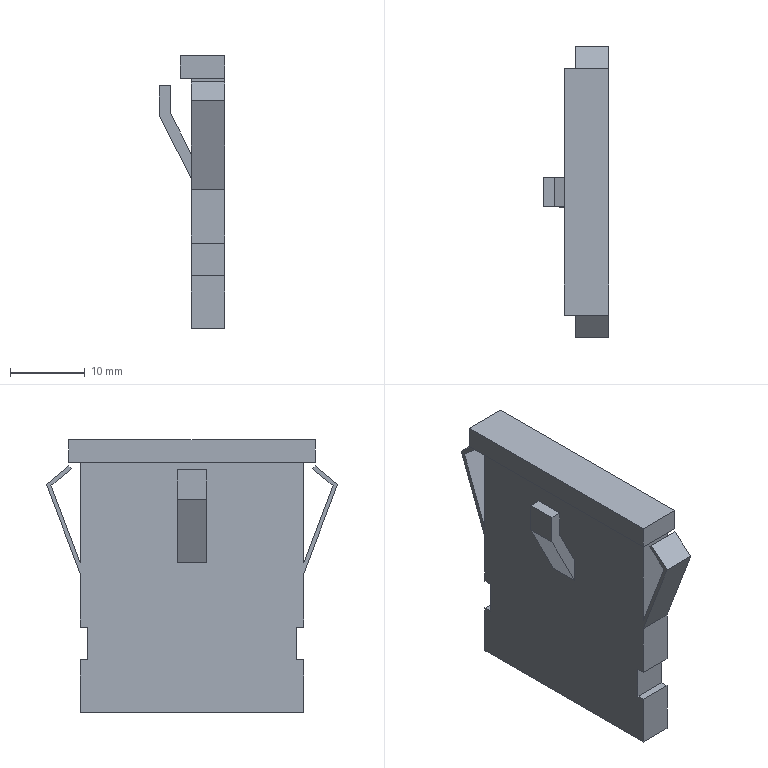Part | STEP file | A7P_M_LEFT | 1 solid | 37 faces | box 8.8 x 39 x 36.5 mm | volume 5217 mm3 | plane 37
STEP:
#1=CARTESIAN_POINT('',(0.,-15.,-26.5));
#2=VERTEX_POINT('',#1);
#3=CARTESIAN_POINT('',(-4.5,-15.,-26.5));
#4=VERTEX_POINT('',#3);
#5=CARTESIAN_POINT('',(0.,-15.,-26.5));
#6=DIRECTION('',(-1.,0.,0.));
#7=VECTOR('',#6,1000.);
#8=LINE('',#5,#7);
#9=EDGE_CURVE('',#2,#4,#8,.T.);
#10=ORIENTED_EDGE('',*,*,#9,.T.);
#11=CARTESIAN_POINT('',(-4.5,-15.,-33.5));
#12=VERTEX_POINT('',#11);
#13=CARTESIAN_POINT('',(-4.5,-15.,0.));
#14=DIRECTION('',(0.,0.,-1.));
#15=VECTOR('',#14,1000.);
#16=LINE('',#13,#15);
#17=EDGE_CURVE('',#4,#12,#16,.T.);
#18=ORIENTED_EDGE('',*,*,#17,.T.);
#19=CARTESIAN_POINT('',(0.,-15.,-33.5));
#20=VERTEX_POINT('',#19);
#21=CARTESIAN_POINT('',(-4.5,-15.,-33.5));
#22=DIRECTION('',(1.,0.,0.));
#23=VECTOR('',#22,1000.);
#24=LINE('',#21,#23);
#25=EDGE_CURVE('',#12,#20,#24,.T.);
#26=ORIENTED_EDGE('',*,*,#25,.T.);
#27=CARTESIAN_POINT('',(0.,-15.,0.));
#28=DIRECTION('',(0.,0.,-1.));
#29=VECTOR('',#28,1000.);
#30=LINE('',#27,#29);
#31=EDGE_CURVE('',#2,#20,#30,.T.);
#32=ORIENTED_EDGE('',*,*,#31,.F.);
#33=EDGE_LOOP('',(#10,#18,#26,#32));
#34=FACE_OUTER_BOUND('',#33,.T.);
#35=CARTESIAN_POINT('',(-4.5,-15.,0.));
#36=DIRECTION('',(0.,-1.,0.));
#37=DIRECTION('',(0.,0.,-1.));
#38=AXIS2_PLACEMENT_3D('',#35,#36,#37);
#39=PLANE('',#38);
#40=ADVANCED_FACE('',(#34),#39,.T.);
#41=CARTESIAN_POINT('',(0.,15.,-26.5));
#42=VERTEX_POINT('',#41);
#43=CARTESIAN_POINT('',(-4.5,15.,-26.5));
#44=VERTEX_POINT('',#43);
#45=CARTESIAN_POINT('',(0.,15.,-26.5));
#46=DIRECTION('',(-1.,0.,0.));
#47=VECTOR('',#46,1000.);
#48=LINE('',#45,#47);
#49=EDGE_CURVE('',#42,#44,#48,.T.);
#50=ORIENTED_EDGE('',*,*,#49,.F.);
#51=CARTESIAN_POINT('',(0.,15.,-33.5));
#52=VERTEX_POINT('',#51);
#53=CARTESIAN_POINT('',(0.,15.,0.));
#54=DIRECTION('',(0.,0.,1.));
#55=VECTOR('',#54,1000.);
#56=LINE('',#53,#55);
#57=EDGE_CURVE('',#52,#42,#56,.T.);
#58=ORIENTED_EDGE('',*,*,#57,.F.);
#59=CARTESIAN_POINT('',(-4.5,15.,-33.5));
#60=VERTEX_POINT('',#59);
#61=CARTESIAN_POINT('',(-4.5,15.,-33.5));
#62=DIRECTION('',(1.,0.,0.));
#63=VECTOR('',#62,1000.);
#64=LINE('',#61,#63);
#65=EDGE_CURVE('',#60,#52,#64,.T.);
#66=ORIENTED_EDGE('',*,*,#65,.F.);
#67=CARTESIAN_POINT('',(-4.5,15.,0.));
#68=DIRECTION('',(0.,0.,1.));
#69=VECTOR('',#68,1000.);
#70=LINE('',#67,#69);
#71=EDGE_CURVE('',#60,#44,#70,.T.);
#72=ORIENTED_EDGE('',*,*,#71,.T.);
#73=EDGE_LOOP('',(#50,#58,#66,#72));
#74=FACE_OUTER_BOUND('',#73,.T.);
#75=CARTESIAN_POINT('',(-4.5,15.,0.));
#76=DIRECTION('',(0.,1.,0.));
#77=DIRECTION('',(0.,0.,1.));
#78=AXIS2_PLACEMENT_3D('',#75,#76,#77);
#79=PLANE('',#78);
#80=ADVANCED_FACE('',(#74),#79,.T.);
#81=CARTESIAN_POINT('',(0.,-15.,-22.1));
#82=VERTEX_POINT('',#81);
#83=CARTESIAN_POINT('',(-4.5,-15.,-22.1));
#84=VERTEX_POINT('',#83);
#85=CARTESIAN_POINT('',(0.,-15.,-22.1));
#86=DIRECTION('',(-1.,0.,0.));
#87=VECTOR('',#86,1000.);
#88=LINE('',#85,#87);
#89=EDGE_CURVE('',#82,#84,#88,.T.);
#90=ORIENTED_EDGE('',*,*,#89,.F.);
#91=CARTESIAN_POINT('',(0.,-15.,-14.9));
#92=VERTEX_POINT('',#91);
#93=CARTESIAN_POINT('',(0.,-15.,0.));
#94=DIRECTION('',(0.,0.,-1.));
#95=VECTOR('',#94,1000.);
#96=LINE('',#93,#95);
#97=EDGE_CURVE('',#92,#82,#96,.T.);
#98=ORIENTED_EDGE('',*,*,#97,.F.);
#99=CARTESIAN_POINT('',(-4.5,-15.,-14.9));
#100=VERTEX_POINT('',#99);
#101=CARTESIAN_POINT('',(0.,-15.,-14.9));
#102=DIRECTION('',(-1.,0.,0.));
#103=VECTOR('',#102,1000.);
#104=LINE('',#101,#103);
#105=EDGE_CURVE('',#92,#100,#104,.T.);
#106=ORIENTED_EDGE('',*,*,#105,.T.);
#107=CARTESIAN_POINT('',(-4.5,-15.,0.));
#108=DIRECTION('',(0.,0.,-1.));
#109=VECTOR('',#108,1000.);
#110=LINE('',#107,#109);
#111=EDGE_CURVE('',#100,#84,#110,.T.);
#112=ORIENTED_EDGE('',*,*,#111,.T.);
#113=EDGE_LOOP('',(#90,#98,#106,#112));
#114=FACE_OUTER_BOUND('',#113,.T.);
#115=CARTESIAN_POINT('',(-4.5,-15.,0.));
#116=DIRECTION('',(0.,-1.,0.));
#117=DIRECTION('',(0.,0.,-1.));
#118=AXIS2_PLACEMENT_3D('',#115,#116,#117);
#119=PLANE('',#118);
#120=ADVANCED_FACE('',(#114),#119,.T.);
#121=CARTESIAN_POINT('',(0.,15.,-22.1));
#122=VERTEX_POINT('',#121);
#123=CARTESIAN_POINT('',(-4.5,15.,-22.1));
#124=VERTEX_POINT('',#123);
#125=CARTESIAN_POINT('',(0.,15.,-22.1));
#126=DIRECTION('',(-1.,0.,0.));
#127=VECTOR('',#126,1000.);
#128=LINE('',#125,#127);
#129=EDGE_CURVE('',#122,#124,#128,.T.);
#130=ORIENTED_EDGE('',*,*,#129,.T.);
#131=CARTESIAN_POINT('',(-4.5,15.,-14.9));
#132=VERTEX_POINT('',#131);
#133=CARTESIAN_POINT('',(-4.5,15.,0.));
#134=DIRECTION('',(0.,0.,1.));
#135=VECTOR('',#134,1000.);
#136=LINE('',#133,#135);
#137=EDGE_CURVE('',#124,#132,#136,.T.);
#138=ORIENTED_EDGE('',*,*,#137,.T.);
#139=CARTESIAN_POINT('',(0.,15.,-14.9));
#140=VERTEX_POINT('',#139);
#141=CARTESIAN_POINT('',(0.,15.,-14.9));
#142=DIRECTION('',(-1.,0.,0.));
#143=VECTOR('',#142,1000.);
#144=LINE('',#141,#143);
#145=EDGE_CURVE('',#140,#132,#144,.T.);
#146=ORIENTED_EDGE('',*,*,#145,.F.);
#147=CARTESIAN_POINT('',(0.,15.,0.));
#148=DIRECTION('',(0.,0.,1.));
#149=VECTOR('',#148,1000.);
#150=LINE('',#147,#149);
#151=EDGE_CURVE('',#122,#140,#150,.T.);
#152=ORIENTED_EDGE('',*,*,#151,.F.);
#153=EDGE_LOOP('',(#130,#138,#146,#152));
#154=FACE_OUTER_BOUND('',#153,.T.);
#155=CARTESIAN_POINT('',(-4.5,15.,0.));
#156=DIRECTION('',(0.,1.,0.));
#157=DIRECTION('',(0.,0.,1.));
#158=AXIS2_PLACEMENT_3D('',#155,#156,#157);
#159=PLANE('',#158);
#160=ADVANCED_FACE('',(#154),#159,.T.);
#161=CARTESIAN_POINT('',(0.,15.,-13.486));
#162=VERTEX_POINT('',#161);
#163=CARTESIAN_POINT('',(-4.5,15.,-13.486));
#164=VERTEX_POINT('',#163);
#165=CARTESIAN_POINT('',(0.,15.,-13.486));
#166=DIRECTION('',(-1.,0.,0.));
#167=VECTOR('',#166,1000.);
#168=LINE('',#165,#167);
#169=EDGE_CURVE('',#162,#164,#168,.T.);
#170=ORIENTED_EDGE('',*,*,#169,.T.);
#171=CARTESIAN_POINT('',(-4.5,15.,0.));
#172=VERTEX_POINT('',#171);
#173=CARTESIAN_POINT('',(-4.5,15.,0.));
#174=DIRECTION('',(0.,0.,1.));
#175=VECTOR('',#174,1000.);
#176=LINE('',#173,#175);
#177=EDGE_CURVE('',#164,#172,#176,.T.);
#178=ORIENTED_EDGE('',*,*,#177,.T.);
#179=CARTESIAN_POINT('',(0.,15.,0.));
#180=VERTEX_POINT('',#179);
#181=CARTESIAN_POINT('',(-4.5,15.,0.));
#182=DIRECTION('',(1.,0.,0.));
#183=VECTOR('',#182,1000.);
#184=LINE('',#181,#183);
#185=EDGE_CURVE('',#172,#180,#184,.T.);
#186=ORIENTED_EDGE('',*,*,#185,.T.);
#187=CARTESIAN_POINT('',(0.,15.,0.));
#188=DIRECTION('',(0.,0.,1.));
#189=VECTOR('',#188,1000.);
#190=LINE('',#187,#189);
#191=EDGE_CURVE('',#162,#180,#190,.T.);
#192=ORIENTED_EDGE('',*,*,#191,.F.);
#193=EDGE_LOOP('',(#170,#178,#186,#192));
#194=FACE_OUTER_BOUND('',#193,.T.);
#195=CARTESIAN_POINT('',(-4.5,15.,0.));
#196=DIRECTION('',(0.,1.,0.));
#197=DIRECTION('',(0.,0.,1.));
#198=AXIS2_PLACEMENT_3D('',#195,#196,#197);
#199=PLANE('',#198);
#200=ADVANCED_FACE('',(#194),#199,.T.);
#201=CARTESIAN_POINT('',(0.,15.,-33.5));
#202=DIRECTION('',(0.,1.,0.));
#203=VECTOR('',#202,1000.);
#204=LINE('',#201,#203);
#205=EDGE_CURVE('',#20,#52,#204,.T.);
#206=ORIENTED_EDGE('',*,*,#205,.F.);
#207=ORIENTED_EDGE('',*,*,#25,.F.);
#208=CARTESIAN_POINT('',(-4.5,15.,-33.5));
#209=DIRECTION('',(0.,1.,0.));
#210=VECTOR('',#209,1000.);
#211=LINE('',#208,#210);
#212=EDGE_CURVE('',#12,#60,#211,.T.);
#213=ORIENTED_EDGE('',*,*,#212,.T.);
#214=ORIENTED_EDGE('',*,*,#65,.T.);
#215=EDGE_LOOP('',(#206,#207,#213,#214));
#216=FACE_OUTER_BOUND('',#215,.T.);
#217=CARTESIAN_POINT('',(-4.5,15.,-33.5));
#218=DIRECTION('',(0.,0.,-1.));
#219=DIRECTION('',(-1.,0.,0.));
#220=AXIS2_PLACEMENT_3D('',#217,#218,#219);
#221=PLANE('',#220);
#222=ADVANCED_FACE('',(#216),#221,.T.);
#223=CARTESIAN_POINT('',(0.,-15.,-13.486));
#224=VERTEX_POINT('',#223);
#225=CARTESIAN_POINT('',(-4.5,-15.,-13.486));
#226=VERTEX_POINT('',#225);
#227=CARTESIAN_POINT('',(0.,-15.,-13.486));
#228=DIRECTION('',(-1.,0.,0.));
#229=VECTOR('',#228,1000.);
#230=LINE('',#227,#229);
#231=EDGE_CURVE('',#224,#226,#230,.T.);
#232=ORIENTED_EDGE('',*,*,#231,.F.);
#233=CARTESIAN_POINT('',(0.,-15.,0.));
#234=VERTEX_POINT('',#233);
#235=CARTESIAN_POINT('',(0.,-15.,0.));
#236=DIRECTION('',(0.,0.,-1.));
#237=VECTOR('',#236,1000.);
#238=LINE('',#235,#237);
#239=EDGE_CURVE('',#234,#224,#238,.T.);
#240=ORIENTED_EDGE('',*,*,#239,.F.);
#241=CARTESIAN_POINT('',(-4.5,-15.,0.));
#242=VERTEX_POINT('',#241);
#243=CARTESIAN_POINT('',(-4.5,-15.,0.));
#244=DIRECTION('',(1.,0.,0.));
#245=VECTOR('',#244,1000.);
#246=LINE('',#243,#245);
#247=EDGE_CURVE('',#242,#234,#246,.T.);
#248=ORIENTED_EDGE('',*,*,#247,.F.);
#249=CARTESIAN_POINT('',(-4.5,-15.,0.));
#250=DIRECTION('',(0.,0.,-1.));
#251=VECTOR('',#250,1000.);
#252=LINE('',#249,#251);
#253=EDGE_CURVE('',#242,#226,#252,.T.);
#254=ORIENTED_EDGE('',*,*,#253,.T.);
#255=EDGE_LOOP('',(#232,#240,#248,#254));
#256=FACE_OUTER_BOUND('',#255,.T.);
#257=CARTESIAN_POINT('',(-4.5,-15.,0.));
#258=DIRECTION('',(0.,-1.,0.));
#259=DIRECTION('',(0.,0.,-1.));
#260=AXIS2_PLACEMENT_3D('',#257,#258,#259);
#261=PLANE('',#260);
#262=ADVANCED_FACE('',(#256),#261,.T.);
#263=CARTESIAN_POINT('',(0.,-16.5,0.));
#264=VERTEX_POINT('',#263);
#265=CARTESIAN_POINT('',(0.,-16.5,0.));
#266=DIRECTION('',(0.,1.,0.));
#267=VECTOR('',#266,1000.);
#268=LINE('',#265,#267);
#269=EDGE_CURVE('',#264,#234,#268,.T.);
#270=ORIENTED_EDGE('',*,*,#269,.F.);
#271=CARTESIAN_POINT('',(-6.,-16.5,0.));
#272=VERTEX_POINT('',#271);
#273=CARTESIAN_POINT('',(-4.5,-16.5,0.));
#274=DIRECTION('',(1.,0.,0.));
#275=VECTOR('',#274,1000.);
#276=LINE('',#273,#275);
#277=EDGE_CURVE('',#272,#264,#276,.T.);
#278=ORIENTED_EDGE('',*,*,#277,.F.);
#279=CARTESIAN_POINT('',(-6.,16.5,0.));
#280=VERTEX_POINT('',#279);
#281=CARTESIAN_POINT('',(-6.,16.5,0.));
#282=DIRECTION('',(0.,-1.,0.));
#283=VECTOR('',#282,1000.);
#284=LINE('',#281,#283);
#285=EDGE_CURVE('',#280,#272,#284,.T.);
#286=ORIENTED_EDGE('',*,*,#285,.F.);
#287=CARTESIAN_POINT('',(0.,16.5,0.));
#288=VERTEX_POINT('',#287);
#289=CARTESIAN_POINT('',(-4.5,16.5,0.));
#290=DIRECTION('',(1.,0.,0.));
#291=VECTOR('',#290,1000.);
#292=LINE('',#289,#291);
#293=EDGE_CURVE('',#280,#288,#292,.T.);
#294=ORIENTED_EDGE('',*,*,#293,.T.);
#295=CARTESIAN_POINT('',(0.,15.,0.));
#296=DIRECTION('',(0.,1.,0.));
#297=VECTOR('',#296,1000.);
#298=LINE('',#295,#297);
#299=EDGE_CURVE('',#180,#288,#298,.T.);
#300=ORIENTED_EDGE('',*,*,#299,.F.);
#301=ORIENTED_EDGE('',*,*,#185,.F.);
#302=CARTESIAN_POINT('',(-4.5,16.5,0.));
#303=DIRECTION('',(0.,1.,0.));
#304=VECTOR('',#303,1000.);
#305=LINE('',#302,#304);
#306=EDGE_CURVE('',#242,#172,#305,.T.);
#307=ORIENTED_EDGE('',*,*,#306,.F.);
#308=ORIENTED_EDGE('',*,*,#247,.T.);
#309=EDGE_LOOP('',(#270,#278,#286,#294,#300,#301,#307,#308));
#310=FACE_OUTER_BOUND('',#309,.T.);
#311=CARTESIAN_POINT('',(-4.5,-16.5,0.));
#312=DIRECTION('',(0.,0.,-1.));
#313=DIRECTION('',(-1.,0.,0.));
#314=AXIS2_PLACEMENT_3D('',#311,#312,#313);
#315=PLANE('',#314);
#316=ADVANCED_FACE('',(#310),#315,.T.);
#317=CARTESIAN_POINT('',(0.,-16.5,3.));
#318=VERTEX_POINT('',#317);
#319=CARTESIAN_POINT('',(0.,-16.5,3.));
#320=DIRECTION('',(0.,0.,-1.));
#321=VECTOR('',#320,1000.);
#322=LINE('',#319,#321);
#323=EDGE_CURVE('',#318,#264,#322,.T.);
#324=ORIENTED_EDGE('',*,*,#323,.F.);
#325=CARTESIAN_POINT('',(-6.,-16.5,3.));
#326=VERTEX_POINT('',#325);
#327=CARTESIAN_POINT('',(-4.5,-16.5,3.));
#328=DIRECTION('',(1.,0.,0.));
#329=VECTOR('',#328,1000.);
#330=LINE('',#327,#329);
#331=EDGE_CURVE('',#326,#318,#330,.T.);
#332=ORIENTED_EDGE('',*,*,#331,.F.);
#333=CARTESIAN_POINT('',(-6.,-16.5,-33.541));
#334=DIRECTION('',(0.,0.,1.));
#335=VECTOR('',#334,1000.);
#336=LINE('',#333,#335);
#337=EDGE_CURVE('',#272,#326,#336,.T.);
#338=ORIENTED_EDGE('',*,*,#337,.F.);
#339=ORIENTED_EDGE('',*,*,#277,.T.);
#340=EDGE_LOOP('',(#324,#332,#338,#339));
#341=FACE_OUTER_BOUND('',#340,.T.);
#342=CARTESIAN_POINT('',(-4.5,-16.5,3.));
#343=DIRECTION('',(0.,-1.,0.));
#344=DIRECTION('',(0.,0.,-1.));
#345=AXIS2_PLACEMENT_3D('',#342,#343,#344);
#346=PLANE('',#345);
#347=ADVANCED_FACE('',(#341),#346,.T.);
#348=CARTESIAN_POINT('',(0.,16.5,3.));
#349=VERTEX_POINT('',#348);
#350=CARTESIAN_POINT('',(0.,16.5,3.));
#351=DIRECTION('',(0.,-1.,0.));
#352=VECTOR('',#351,1000.);
#353=LINE('',#350,#352);
#354=EDGE_CURVE('',#349,#318,#353,.T.);
#355=ORIENTED_EDGE('',*,*,#354,.F.);
#356=CARTESIAN_POINT('',(-6.,16.5,3.));
#357=VERTEX_POINT('',#356);
#358=CARTESIAN_POINT('',(-4.5,16.5,3.));
#359=DIRECTION('',(1.,0.,0.));
#360=VECTOR('',#359,1000.);
#361=LINE('',#358,#360);
#362=EDGE_CURVE('',#357,#349,#361,.T.);
#363=ORIENTED_EDGE('',*,*,#362,.F.);
#364=CARTESIAN_POINT('',(-6.,16.5,3.));
#365=DIRECTION('',(0.,-1.,0.));
#366=VECTOR('',#365,1000.);
#367=LINE('',#364,#366);
#368=EDGE_CURVE('',#357,#326,#367,.T.);
#369=ORIENTED_EDGE('',*,*,#368,.T.);
#370=ORIENTED_EDGE('',*,*,#331,.T.);
#371=EDGE_LOOP('',(#355,#363,#369,#370));
#372=FACE_OUTER_BOUND('',#371,.T.);
#373=CARTESIAN_POINT('',(-4.5,16.5,3.));
#374=DIRECTION('',(0.,0.,1.));
#375=DIRECTION('',(1.,0.,0.));
#376=AXIS2_PLACEMENT_3D('',#373,#374,#375);
#377=PLANE('',#376);
#378=ADVANCED_FACE('',(#372),#377,.T.);
#379=CARTESIAN_POINT('',(0.,16.5,0.));
#380=DIRECTION('',(0.,0.,1.));
#381=VECTOR('',#380,1000.);
#382=LINE('',#379,#381);
#383=EDGE_CURVE('',#288,#349,#382,.T.);
#384=ORIENTED_EDGE('',*,*,#383,.F.);
#385=ORIENTED_EDGE('',*,*,#293,.F.);
#386=CARTESIAN_POINT('',(-6.,16.5,-33.541));
#387=DIRECTION('',(0.,0.,1.));
#388=VECTOR('',#387,1000.);
#389=LINE('',#386,#388);
#390=EDGE_CURVE('',#280,#357,#389,.T.);
#391=ORIENTED_EDGE('',*,*,#390,.T.);
#392=ORIENTED_EDGE('',*,*,#362,.T.);
#393=EDGE_LOOP('',(#384,#385,#391,#392));
#394=FACE_OUTER_BOUND('',#393,.T.);
#395=CARTESIAN_POINT('',(-4.5,16.5,0.));
#396=DIRECTION('',(0.,1.,0.));
#397=DIRECTION('',(0.,0.,1.));
#398=AXIS2_PLACEMENT_3D('',#395,#396,#397);
#399=PLANE('',#398);
#400=ADVANCED_FACE('',(#394),#399,.T.);
#401=CARTESIAN_POINT('',(-4.5,2.,-13.5));
#402=VERTEX_POINT('',#401);
#403=CARTESIAN_POINT('',(-4.5,-2.,-13.5));
#404=VERTEX_POINT('',#403);
#405=CARTESIAN_POINT('',(-4.5,2.,-13.5));
#406=DIRECTION('',(0.,-1.,0.));
#407=VECTOR('',#406,1000.);
#408=LINE('',#405,#407);
#409=EDGE_CURVE('',#402,#404,#408,.T.);
#410=ORIENTED_EDGE('',*,*,#409,.F.);
#411=CARTESIAN_POINT('',(-4.5,2.,-10.177));
#412=VERTEX_POINT('',#411);
#413=CARTESIAN_POINT('',(-4.5,2.,-13.5));
#414=DIRECTION('',(0.,0.,-1.));
#415=VECTOR('',#414,1000.);
#416=LINE('',#413,#415);
#417=EDGE_CURVE('',#412,#402,#416,.T.);
#418=ORIENTED_EDGE('',*,*,#417,.F.);
#419=CARTESIAN_POINT('',(-4.5,-2.,-10.177));
#420=VERTEX_POINT('',#419);
#421=CARTESIAN_POINT('',(-4.5,2.,-10.177));
#422=DIRECTION('',(0.,-1.,0.));
#423=VECTOR('',#422,1000.);
#424=LINE('',#421,#423);
#425=EDGE_CURVE('',#412,#420,#424,.T.);
#426=ORIENTED_EDGE('',*,*,#425,.T.);
#427=CARTESIAN_POINT('',(-4.5,-2.,-13.5));
#428=DIRECTION('',(0.,0.,-1.));
#429=VECTOR('',#428,1000.);
#430=LINE('',#427,#429);
#431=EDGE_CURVE('',#420,#404,#430,.T.);
#432=ORIENTED_EDGE('',*,*,#431,.T.);
#433=EDGE_LOOP('',(#410,#418,#426,#432));
#434=FACE_BOUND('',#433,.T.);
#435=ORIENTED_EDGE('',*,*,#17,.F.);
#436=CARTESIAN_POINT('',(-4.5,-14.,-26.5));
#437=VERTEX_POINT('',#436);
#438=CARTESIAN_POINT('',(-4.5,-15.,-26.5));
#439=DIRECTION('',(0.,-1.,0.));
#440=VECTOR('',#439,1000.);
#441=LINE('',#438,#440);
#442=EDGE_CURVE('',#437,#4,#441,.T.);
#443=ORIENTED_EDGE('',*,*,#442,.F.);
#444=CARTESIAN_POINT('',(-4.5,-14.,-22.1));
#445=VERTEX_POINT('',#444);
#446=CARTESIAN_POINT('',(-4.5,-14.,-26.5));
#447=DIRECTION('',(0.,0.,-1.));
#448=VECTOR('',#447,1000.);
#449=LINE('',#446,#448);
#450=EDGE_CURVE('',#445,#437,#449,.T.);
#451=ORIENTED_EDGE('',*,*,#450,.F.);
#452=CARTESIAN_POINT('',(-4.5,-15.,-22.1));
#453=DIRECTION('',(0.,1.,0.));
#454=VECTOR('',#453,1000.);
#455=LINE('',#452,#454);
#456=EDGE_CURVE('',#84,#445,#455,.T.);
#457=ORIENTED_EDGE('',*,*,#456,.F.);
#458=ORIENTED_EDGE('',*,*,#111,.F.);
#459=CARTESIAN_POINT('',(-4.5,-19.5,-3.));
#460=VERTEX_POINT('',#459);
#461=CARTESIAN_POINT('',(-4.5,-15.,-14.9));
#462=DIRECTION('',(0.,-0.3537,0.9354));
#463=VECTOR('',#462,1000.);
#464=LINE('',#461,#463);
#465=EDGE_CURVE('',#100,#460,#464,.T.);
#466=ORIENTED_EDGE('',*,*,#465,.T.);
#467=CARTESIAN_POINT('',(-4.5,-16.5,-0.5));
#468=VERTEX_POINT('',#467);
#469=CARTESIAN_POINT('',(-4.5,-19.5,-3.));
#470=DIRECTION('',(0.,0.7682,0.6402));
#471=VECTOR('',#470,1000.);
#472=LINE('',#469,#471);
#473=EDGE_CURVE('',#460,#468,#472,.T.);
#474=ORIENTED_EDGE('',*,*,#473,.T.);
#475=CARTESIAN_POINT('',(-4.5,-16.18,-0.8841));
#476=VERTEX_POINT('',#475);
#477=CARTESIAN_POINT('',(-4.5,-16.5,-0.5));
#478=DIRECTION('',(0.,0.6402,-0.7682));
#479=VECTOR('',#478,1000.);
#480=LINE('',#477,#479);
#481=EDGE_CURVE('',#468,#476,#480,.T.);
#482=ORIENTED_EDGE('',*,*,#481,.T.);
#483=CARTESIAN_POINT('',(-4.5,-18.906,-3.156));
#484=VERTEX_POINT('',#483);
#485=CARTESIAN_POINT('',(-4.5,-18.906,-3.156));
#486=DIRECTION('',(0.,-0.7682,-0.6402));
#487=VECTOR('',#486,1000.);
#488=LINE('',#485,#487);
#489=EDGE_CURVE('',#476,#484,#488,.T.);
#490=ORIENTED_EDGE('',*,*,#489,.T.);
#491=CARTESIAN_POINT('',(-4.5,-15.,-13.486));
#492=DIRECTION('',(0.,0.3537,-0.9354));
#493=VECTOR('',#492,1000.);
#494=LINE('',#491,#493);
#495=EDGE_CURVE('',#484,#226,#494,.T.);
#496=ORIENTED_EDGE('',*,*,#495,.T.);
#497=ORIENTED_EDGE('',*,*,#253,.F.);
#498=ORIENTED_EDGE('',*,*,#306,.T.);
#499=ORIENTED_EDGE('',*,*,#177,.F.);
#500=CARTESIAN_POINT('',(-4.5,18.906,-3.156));
#501=VERTEX_POINT('',#500);
#502=CARTESIAN_POINT('',(-4.5,15.,-13.486));
#503=DIRECTION('',(0.,0.3537,0.9354));
#504=VECTOR('',#503,1000.);
#505=LINE('',#502,#504);
#506=EDGE_CURVE('',#164,#501,#505,.T.);
#507=ORIENTED_EDGE('',*,*,#506,.T.);
#508=CARTESIAN_POINT('',(-4.5,16.18,-0.8841));
#509=VERTEX_POINT('',#508);
#510=CARTESIAN_POINT('',(-4.5,18.906,-3.156));
#511=DIRECTION('',(0.,-0.7682,0.6402));
#512=VECTOR('',#511,1000.);
#513=LINE('',#510,#512);
#514=EDGE_CURVE('',#501,#509,#513,.T.);
#515=ORIENTED_EDGE('',*,*,#514,.T.);
#516=CARTESIAN_POINT('',(-4.5,16.5,-0.5));
#517=VERTEX_POINT('',#516);
#518=CARTESIAN_POINT('',(-4.5,16.5,-0.5));
#519=DIRECTION('',(0.,0.6402,0.7682));
#520=VECTOR('',#519,1000.);
#521=LINE('',#518,#520);
#522=EDGE_CURVE('',#509,#517,#521,.T.);
#523=ORIENTED_EDGE('',*,*,#522,.T.);
#524=CARTESIAN_POINT('',(-4.5,19.5,-3.));
#525=VERTEX_POINT('',#524);
#526=CARTESIAN_POINT('',(-4.5,19.5,-3.));
#527=DIRECTION('',(0.,0.7682,-0.6402));
#528=VECTOR('',#527,1000.);
#529=LINE('',#526,#528);
#530=EDGE_CURVE('',#517,#525,#529,.T.);
#531=ORIENTED_EDGE('',*,*,#530,.T.);
#532=CARTESIAN_POINT('',(-4.5,15.,-14.9));
#533=DIRECTION('',(0.,-0.3537,-0.9354));
#534=VECTOR('',#533,1000.);
#535=LINE('',#532,#534);
#536=EDGE_CURVE('',#525,#132,#535,.T.);
#537=ORIENTED_EDGE('',*,*,#536,.T.);
#538=ORIENTED_EDGE('',*,*,#137,.F.);
#539=CARTESIAN_POINT('',(-4.5,14.,-22.1));
#540=VERTEX_POINT('',#539);
#541=CARTESIAN_POINT('',(-4.5,15.,-22.1));
#542=DIRECTION('',(0.,1.,0.));
#543=VECTOR('',#542,1000.);
#544=LINE('',#541,#543);
#545=EDGE_CURVE('',#540,#124,#544,.T.);
#546=ORIENTED_EDGE('',*,*,#545,.F.);
#547=CARTESIAN_POINT('',(-4.5,14.,-26.5));
#548=VERTEX_POINT('',#547);
#549=CARTESIAN_POINT('',(-4.5,14.,-26.5));
#550=DIRECTION('',(0.,0.,1.));
#551=VECTOR('',#550,1000.);
#552=LINE('',#549,#551);
#553=EDGE_CURVE('',#548,#540,#552,.T.);
#554=ORIENTED_EDGE('',*,*,#553,.F.);
#555=CARTESIAN_POINT('',(-4.5,15.,-26.5));
#556=DIRECTION('',(0.,-1.,0.));
#557=VECTOR('',#556,1000.);
#558=LINE('',#555,#557);
#559=EDGE_CURVE('',#44,#548,#558,.T.);
#560=ORIENTED_EDGE('',*,*,#559,.F.);
#561=ORIENTED_EDGE('',*,*,#71,.F.);
#562=ORIENTED_EDGE('',*,*,#212,.F.);
#563=EDGE_LOOP('',(#435,#443,#451,#457,#458,#466,#474,#482,#490,#496,#497,#498,#499,#507,#515,#523,#531,#537,#538,#546,#554,#560,#561,#562));
#564=FACE_OUTER_BOUND('',#563,.T.);
#565=CARTESIAN_POINT('',(-4.5,16.5,0.));
#566=DIRECTION('',(1.,0.,0.));
#567=DIRECTION('',(0.,0.,-1.));
#568=AXIS2_PLACEMENT_3D('',#565,#566,#567);
#569=PLANE('',#568);
#570=ADVANCED_FACE('',(#434,#564),#569,.F.);
#571=CARTESIAN_POINT('',(0.,-14.,-26.5));
#572=VERTEX_POINT('',#571);
#573=CARTESIAN_POINT('',(0.,-15.,-26.5));
#574=DIRECTION('',(0.,-1.,0.));
#575=VECTOR('',#574,1000.);
#576=LINE('',#573,#575);
#577=EDGE_CURVE('',#572,#2,#576,.T.);
#578=ORIENTED_EDGE('',*,*,#577,.T.);
#579=ORIENTED_EDGE('',*,*,#31,.T.);
#580=ORIENTED_EDGE('',*,*,#205,.T.);
#581=ORIENTED_EDGE('',*,*,#57,.T.);
#582=CARTESIAN_POINT('',(0.,14.,-26.5));
#583=VERTEX_POINT('',#582);
#584=CARTESIAN_POINT('',(0.,15.,-26.5));
#585=DIRECTION('',(0.,-1.,0.));
#586=VECTOR('',#585,1000.);
#587=LINE('',#584,#586);
#588=EDGE_CURVE('',#42,#583,#587,.T.);
#589=ORIENTED_EDGE('',*,*,#588,.T.);
#590=CARTESIAN_POINT('',(0.,14.,-22.1));
#591=VERTEX_POINT('',#590);
#592=CARTESIAN_POINT('',(0.,14.,-26.5));
#593=DIRECTION('',(0.,0.,1.));
#594=VECTOR('',#593,1000.);
#595=LINE('',#592,#594);
#596=EDGE_CURVE('',#583,#591,#595,.T.);
#597=ORIENTED_EDGE('',*,*,#596,.T.);
#598=CARTESIAN_POINT('',(0.,15.,-22.1));
#599=DIRECTION('',(0.,1.,0.));
#600=VECTOR('',#599,1000.);
#601=LINE('',#598,#600);
#602=EDGE_CURVE('',#591,#122,#601,.T.);
#603=ORIENTED_EDGE('',*,*,#602,.T.);
#604=ORIENTED_EDGE('',*,*,#151,.T.);
#605=CARTESIAN_POINT('',(0.,19.5,-3.));
#606=VERTEX_POINT('',#605);
#607=CARTESIAN_POINT('',(0.,15.,-14.9));
#608=DIRECTION('',(0.,-0.3537,-0.9354));
#609=VECTOR('',#608,1000.);
#610=LINE('',#607,#609);
#611=EDGE_CURVE('',#606,#140,#610,.T.);
#612=ORIENTED_EDGE('',*,*,#611,.F.);
#613=CARTESIAN_POINT('',(0.,16.5,-0.5));
#614=VERTEX_POINT('',#613);
#615=CARTESIAN_POINT('',(0.,19.5,-3.));
#616=DIRECTION('',(0.,0.7682,-0.6402));
#617=VECTOR('',#616,1000.);
#618=LINE('',#615,#617);
#619=EDGE_CURVE('',#614,#606,#618,.T.);
#620=ORIENTED_EDGE('',*,*,#619,.F.);
#621=CARTESIAN_POINT('',(0.,16.18,-0.8841));
#622=VERTEX_POINT('',#621);
#623=CARTESIAN_POINT('',(0.,16.5,-0.5));
#624=DIRECTION('',(0.,0.6402,0.7682));
#625=VECTOR('',#624,1000.);
#626=LINE('',#623,#625);
#627=EDGE_CURVE('',#622,#614,#626,.T.);
#628=ORIENTED_EDGE('',*,*,#627,.F.);
#629=CARTESIAN_POINT('',(0.,18.906,-3.156));
#630=VERTEX_POINT('',#629);
#631=CARTESIAN_POINT('',(0.,18.906,-3.156));
#632=DIRECTION('',(0.,-0.7682,0.6402));
#633=VECTOR('',#632,1000.);
#634=LINE('',#631,#633);
#635=EDGE_CURVE('',#630,#622,#634,.T.);
#636=ORIENTED_EDGE('',*,*,#635,.F.);
#637=CARTESIAN_POINT('',(0.,15.,-13.486));
#638=DIRECTION('',(0.,0.3537,0.9354));
#639=VECTOR('',#638,1000.);
#640=LINE('',#637,#639);
#641=EDGE_CURVE('',#162,#630,#640,.T.);
#642=ORIENTED_EDGE('',*,*,#641,.F.);
#643=ORIENTED_EDGE('',*,*,#191,.T.);
#644=ORIENTED_EDGE('',*,*,#299,.T.);
#645=ORIENTED_EDGE('',*,*,#383,.T.);
#646=ORIENTED_EDGE('',*,*,#354,.T.);
#647=ORIENTED_EDGE('',*,*,#323,.T.);
#648=ORIENTED_EDGE('',*,*,#269,.T.);
#649=ORIENTED_EDGE('',*,*,#239,.T.);
#650=CARTESIAN_POINT('',(0.,-18.906,-3.156));
#651=VERTEX_POINT('',#650);
#652=CARTESIAN_POINT('',(0.,-15.,-13.486));
#653=DIRECTION('',(0.,0.3537,-0.9354));
#654=VECTOR('',#653,1000.);
#655=LINE('',#652,#654);
#656=EDGE_CURVE('',#651,#224,#655,.T.);
#657=ORIENTED_EDGE('',*,*,#656,.F.);
#658=CARTESIAN_POINT('',(0.,-16.18,-0.8841));
#659=VERTEX_POINT('',#658);
#660=CARTESIAN_POINT('',(0.,-18.906,-3.156));
#661=DIRECTION('',(0.,-0.7682,-0.6402));
#662=VECTOR('',#661,1000.);
#663=LINE('',#660,#662);
#664=EDGE_CURVE('',#659,#651,#663,.T.);
#665=ORIENTED_EDGE('',*,*,#664,.F.);
#666=CARTESIAN_POINT('',(0.,-16.5,-0.5));
#667=VERTEX_POINT('',#666);
#668=CARTESIAN_POINT('',(0.,-16.5,-0.5));
#669=DIRECTION('',(0.,0.6402,-0.7682));
#670=VECTOR('',#669,1000.);
#671=LINE('',#668,#670);
#672=EDGE_CURVE('',#667,#659,#671,.T.);
#673=ORIENTED_EDGE('',*,*,#672,.F.);
#674=CARTESIAN_POINT('',(0.,-19.5,-3.));
#675=VERTEX_POINT('',#674);
#676=CARTESIAN_POINT('',(0.,-19.5,-3.));
#677=DIRECTION('',(0.,0.7682,0.6402));
#678=VECTOR('',#677,1000.);
#679=LINE('',#676,#678);
#680=EDGE_CURVE('',#675,#667,#679,.T.);
#681=ORIENTED_EDGE('',*,*,#680,.F.);
#682=CARTESIAN_POINT('',(0.,-15.,-14.9));
#683=DIRECTION('',(0.,-0.3537,0.9354));
#684=VECTOR('',#683,1000.);
#685=LINE('',#682,#684);
#686=EDGE_CURVE('',#92,#675,#685,.T.);
#687=ORIENTED_EDGE('',*,*,#686,.F.);
#688=ORIENTED_EDGE('',*,*,#97,.T.);
#689=CARTESIAN_POINT('',(0.,-14.,-22.1));
#690=VERTEX_POINT('',#689);
#691=CARTESIAN_POINT('',(0.,-15.,-22.1));
#692=DIRECTION('',(0.,1.,0.));
#693=VECTOR('',#692,1000.);
#694=LINE('',#691,#693);
#695=EDGE_CURVE('',#82,#690,#694,.T.);
#696=ORIENTED_EDGE('',*,*,#695,.T.);
#697=CARTESIAN_POINT('',(0.,-14.,-26.5));
#698=DIRECTION('',(0.,0.,-1.));
#699=VECTOR('',#698,1000.);
#700=LINE('',#697,#699);
#701=EDGE_CURVE('',#690,#572,#700,.T.);
#702=ORIENTED_EDGE('',*,*,#701,.T.);
#703=EDGE_LOOP('',(#578,#579,#580,#581,#589,#597,#603,#604,#612,#620,#628,#636,#642,#643,#644,#645,#646,#647,#648,#649,#657,#665,#673,#681,#687,#688,#696,#702));
#704=FACE_OUTER_BOUND('',#703,.T.);
#705=CARTESIAN_POINT('',(0.,16.5,0.));
#706=DIRECTION('',(1.,0.,0.));
#707=DIRECTION('',(0.,0.,-1.));
#708=AXIS2_PLACEMENT_3D('',#705,#706,#707);
#709=PLANE('',#708);
#710=ADVANCED_FACE('',(#704),#709,.T.);
#711=ORIENTED_EDGE('',*,*,#390,.F.);
#712=ORIENTED_EDGE('',*,*,#285,.T.);
#713=ORIENTED_EDGE('',*,*,#337,.T.);
#714=ORIENTED_EDGE('',*,*,#368,.F.);
#715=EDGE_LOOP('',(#711,#712,#713,#714));
#716=FACE_OUTER_BOUND('',#715,.T.);
#717=CARTESIAN_POINT('',(-6.,16.5,-33.541));
#718=DIRECTION('',(-1.,0.,0.));
#719=DIRECTION('',(0.,-1.,0.));
#720=AXIS2_PLACEMENT_3D('',#717,#718,#719);
#721=PLANE('',#720);
#722=ADVANCED_FACE('',(#716),#721,.T.);
#723=CARTESIAN_POINT('',(-8.8,-2.,-5.));
#724=VERTEX_POINT('',#723);
#725=CARTESIAN_POINT('',(-4.5,-2.,-13.5));
#726=DIRECTION('',(-0.4514,0.,0.8923));
#727=VECTOR('',#726,1000.);
#728=LINE('',#725,#727);
#729=EDGE_CURVE('',#404,#724,#728,.T.);
#730=ORIENTED_EDGE('',*,*,#729,.T.);
#731=CARTESIAN_POINT('',(-8.8,2.,-5.));
#732=VERTEX_POINT('',#731);
#733=CARTESIAN_POINT('',(-8.8,2.,-5.));
#734=DIRECTION('',(0.,-1.,0.));
#735=VECTOR('',#734,1000.);
#736=LINE('',#733,#735);
#737=EDGE_CURVE('',#732,#724,#736,.T.);
#738=ORIENTED_EDGE('',*,*,#737,.F.);
#739=CARTESIAN_POINT('',(-4.5,2.,-13.5));
#740=DIRECTION('',(-0.4514,0.,0.8923));
#741=VECTOR('',#740,1000.);
#742=LINE('',#739,#741);
#743=EDGE_CURVE('',#402,#732,#742,.T.);
#744=ORIENTED_EDGE('',*,*,#743,.F.);
#745=ORIENTED_EDGE('',*,*,#409,.T.);
#746=EDGE_LOOP('',(#730,#738,#744,#745));
#747=FACE_OUTER_BOUND('',#746,.T.);
#748=CARTESIAN_POINT('',(-4.5,2.,-13.5));
#749=DIRECTION('',(0.8923,0.,0.4514));
#750=DIRECTION('',(0.4514,0.,-0.8923));
#751=AXIS2_PLACEMENT_3D('',#748,#749,#750);
#752=PLANE('',#751);
#753=ADVANCED_FACE('',(#747),#752,.F.);
#754=CARTESIAN_POINT('',(-8.8,-2.,-1.));
#755=VERTEX_POINT('',#754);
#756=CARTESIAN_POINT('',(-8.8,-2.,-5.));
#757=DIRECTION('',(0.,0.,1.));
#758=VECTOR('',#757,1000.);
#759=LINE('',#756,#758);
#760=EDGE_CURVE('',#724,#755,#759,.T.);
#761=ORIENTED_EDGE('',*,*,#760,.T.);
#762=CARTESIAN_POINT('',(-8.8,2.,-1.));
#763=VERTEX_POINT('',#762);
#764=CARTESIAN_POINT('',(-8.8,2.,-1.));
#765=DIRECTION('',(0.,-1.,0.));
#766=VECTOR('',#765,1000.);
#767=LINE('',#764,#766);
#768=EDGE_CURVE('',#763,#755,#767,.T.);
#769=ORIENTED_EDGE('',*,*,#768,.F.);
#770=CARTESIAN_POINT('',(-8.8,2.,-5.));
#771=DIRECTION('',(0.,0.,1.));
#772=VECTOR('',#771,1000.);
#773=LINE('',#770,#772);
#774=EDGE_CURVE('',#732,#763,#773,.T.);
#775=ORIENTED_EDGE('',*,*,#774,.F.);
#776=ORIENTED_EDGE('',*,*,#737,.T.);
#777=EDGE_LOOP('',(#761,#769,#775,#776));
#778=FACE_OUTER_BOUND('',#777,.T.);
#779=CARTESIAN_POINT('',(-8.8,2.,-5.));
#780=DIRECTION('',(1.,0.,0.));
#781=DIRECTION('',(0.,0.,-1.));
#782=AXIS2_PLACEMENT_3D('',#779,#780,#781);
#783=PLANE('',#782);
#784=ADVANCED_FACE('',(#778),#783,.F.);
#785=CARTESIAN_POINT('',(-7.3,-2.,-1.));
#786=VERTEX_POINT('',#785);
#787=CARTESIAN_POINT('',(-8.8,-2.,-1.));
#788=DIRECTION('',(1.,0.,0.));
#789=VECTOR('',#788,1000.);
#790=LINE('',#787,#789);
#791=EDGE_CURVE('',#755,#786,#790,.T.);
#792=ORIENTED_EDGE('',*,*,#791,.T.);
#793=CARTESIAN_POINT('',(-7.3,2.,-1.));
#794=VERTEX_POINT('',#793);
#795=CARTESIAN_POINT('',(-7.3,2.,-1.));
#796=DIRECTION('',(0.,-1.,0.));
#797=VECTOR('',#796,1000.);
#798=LINE('',#795,#797);
#799=EDGE_CURVE('',#794,#786,#798,.T.);
#800=ORIENTED_EDGE('',*,*,#799,.F.);
#801=CARTESIAN_POINT('',(-8.8,2.,-1.));
#802=DIRECTION('',(1.,0.,0.));
#803=VECTOR('',#802,1000.);
#804=LINE('',#801,#803);
#805=EDGE_CURVE('',#763,#794,#804,.T.);
#806=ORIENTED_EDGE('',*,*,#805,.F.);
#807=ORIENTED_EDGE('',*,*,#768,.T.);
#808=EDGE_LOOP('',(#792,#800,#806,#807));
#809=FACE_OUTER_BOUND('',#808,.T.);
#810=CARTESIAN_POINT('',(-8.8,2.,-1.));
#811=DIRECTION('',(0.,0.,-1.));
#812=DIRECTION('',(-1.,0.,0.));
#813=AXIS2_PLACEMENT_3D('',#810,#811,#812);
#814=PLANE('',#813);
#815=ADVANCED_FACE('',(#809),#814,.F.);
#816=CARTESIAN_POINT('',(-7.3,-2.,-4.642));
#817=VERTEX_POINT('',#816);
#818=CARTESIAN_POINT('',(-7.3,-2.,-4.642));
#819=DIRECTION('',(0.,0.,-1.));
#820=VECTOR('',#819,1000.);
#821=LINE('',#818,#820);
#822=EDGE_CURVE('',#786,#817,#821,.T.);
#823=ORIENTED_EDGE('',*,*,#822,.T.);
#824=CARTESIAN_POINT('',(-7.3,2.,-4.642));
#825=VERTEX_POINT('',#824);
#826=CARTESIAN_POINT('',(-7.3,2.,-4.642));
#827=DIRECTION('',(0.,-1.,0.));
#828=VECTOR('',#827,1000.);
#829=LINE('',#826,#828);
#830=EDGE_CURVE('',#825,#817,#829,.T.);
#831=ORIENTED_EDGE('',*,*,#830,.F.);
#832=CARTESIAN_POINT('',(-7.3,2.,-4.642));
#833=DIRECTION('',(0.,0.,-1.));
#834=VECTOR('',#833,1000.);
#835=LINE('',#832,#834);
#836=EDGE_CURVE('',#794,#825,#835,.T.);
#837=ORIENTED_EDGE('',*,*,#836,.F.);
#838=ORIENTED_EDGE('',*,*,#799,.T.);
#839=EDGE_LOOP('',(#823,#831,#837,#838));
#840=FACE_OUTER_BOUND('',#839,.T.);
#841=CARTESIAN_POINT('',(-7.3,2.,-4.642));
#842=DIRECTION('',(-1.,0.,0.));
#843=DIRECTION('',(0.,0.,1.));
#844=AXIS2_PLACEMENT_3D('',#841,#842,#843);
#845=PLANE('',#844);
#846=ADVANCED_FACE('',(#840),#845,.F.);
#847=CARTESIAN_POINT('',(-4.5,-2.,-10.177));
#848=DIRECTION('',(0.4514,0.,-0.8923));
#849=VECTOR('',#848,1000.);
#850=LINE('',#847,#849);
#851=EDGE_CURVE('',#817,#420,#850,.T.);
#852=ORIENTED_EDGE('',*,*,#851,.T.);
#853=ORIENTED_EDGE('',*,*,#425,.F.);
#854=CARTESIAN_POINT('',(-4.5,2.,-10.177));
#855=DIRECTION('',(0.4514,0.,-0.8923));
#856=VECTOR('',#855,1000.);
#857=LINE('',#854,#856);
#858=EDGE_CURVE('',#825,#412,#857,.T.);
#859=ORIENTED_EDGE('',*,*,#858,.F.);
#860=ORIENTED_EDGE('',*,*,#830,.T.);
#861=EDGE_LOOP('',(#852,#853,#859,#860));
#862=FACE_OUTER_BOUND('',#861,.T.);
#863=CARTESIAN_POINT('',(-4.5,2.,-10.177));
#864=DIRECTION('',(-0.8923,0.,-0.4514));
#865=DIRECTION('',(-0.4514,0.,0.8923));
#866=AXIS2_PLACEMENT_3D('',#863,#864,#865);
#867=PLANE('',#866);
#868=ADVANCED_FACE('',(#862),#867,.F.);
#869=ORIENTED_EDGE('',*,*,#417,.T.);
#870=ORIENTED_EDGE('',*,*,#743,.T.);
#871=ORIENTED_EDGE('',*,*,#774,.T.);
#872=ORIENTED_EDGE('',*,*,#805,.T.);
#873=ORIENTED_EDGE('',*,*,#836,.T.);
#874=ORIENTED_EDGE('',*,*,#858,.T.);
#875=EDGE_LOOP('',(#869,#870,#871,#872,#873,#874));
#876=FACE_OUTER_BOUND('',#875,.T.);
#877=CARTESIAN_POINT('',(-4.5,2.,-1.));
#878=DIRECTION('',(0.,1.,0.));
#879=DIRECTION('',(0.,0.,1.));
#880=AXIS2_PLACEMENT_3D('',#877,#878,#879);
#881=PLANE('',#880);
#882=ADVANCED_FACE('',(#876),#881,.T.);
#883=ORIENTED_EDGE('',*,*,#431,.F.);
#884=ORIENTED_EDGE('',*,*,#851,.F.);
#885=ORIENTED_EDGE('',*,*,#822,.F.);
#886=ORIENTED_EDGE('',*,*,#791,.F.);
#887=ORIENTED_EDGE('',*,*,#760,.F.);
#888=ORIENTED_EDGE('',*,*,#729,.F.);
#889=EDGE_LOOP('',(#883,#884,#885,#886,#887,#888));
#890=FACE_OUTER_BOUND('',#889,.T.);
#891=CARTESIAN_POINT('',(-4.5,-2.,-1.));
#892=DIRECTION('',(0.,1.,0.));
#893=DIRECTION('',(0.,0.,1.));
#894=AXIS2_PLACEMENT_3D('',#891,#892,#893);
#895=PLANE('',#894);
#896=ADVANCED_FACE('',(#890),#895,.F.);
#897=ORIENTED_EDGE('',*,*,#536,.F.);
#898=CARTESIAN_POINT('',(0.,19.5,-3.));
#899=DIRECTION('',(-1.,0.,0.));
#900=VECTOR('',#899,1000.);
#901=LINE('',#898,#900);
#902=EDGE_CURVE('',#606,#525,#901,.T.);
#903=ORIENTED_EDGE('',*,*,#902,.F.);
#904=ORIENTED_EDGE('',*,*,#611,.T.);
#905=ORIENTED_EDGE('',*,*,#145,.T.);
#906=EDGE_LOOP('',(#897,#903,#904,#905));
#907=FACE_OUTER_BOUND('',#906,.T.);
#908=CARTESIAN_POINT('',(0.,15.,-14.9));
#909=DIRECTION('',(0.,0.9354,-0.3537));
#910=DIRECTION('',(0.,0.3537,0.9354));
#911=AXIS2_PLACEMENT_3D('',#908,#909,#910);
#912=PLANE('',#911);
#913=ADVANCED_FACE('',(#907),#912,.T.);
#914=ORIENTED_EDGE('',*,*,#530,.F.);
#915=CARTESIAN_POINT('',(0.,16.5,-0.5));
#916=DIRECTION('',(-1.,0.,0.));
#917=VECTOR('',#916,1000.);
#918=LINE('',#915,#917);
#919=EDGE_CURVE('',#614,#517,#918,.T.);
#920=ORIENTED_EDGE('',*,*,#919,.F.);
#921=ORIENTED_EDGE('',*,*,#619,.T.);
#922=ORIENTED_EDGE('',*,*,#902,.T.);
#923=EDGE_LOOP('',(#914,#920,#921,#922));
#924=FACE_OUTER_BOUND('',#923,.T.);
#925=CARTESIAN_POINT('',(0.,19.5,-3.));
#926=DIRECTION('',(0.,0.6402,0.7682));
#927=DIRECTION('',(0.,-0.7682,0.6402));
#928=AXIS2_PLACEMENT_3D('',#925,#926,#927);
#929=PLANE('',#928);
#930=ADVANCED_FACE('',(#924),#929,.T.);
#931=ORIENTED_EDGE('',*,*,#522,.F.);
#932=CARTESIAN_POINT('',(0.,16.18,-0.8841));
#933=DIRECTION('',(-1.,0.,0.));
#934=VECTOR('',#933,1000.);
#935=LINE('',#932,#934);
#936=EDGE_CURVE('',#622,#509,#935,.T.);
#937=ORIENTED_EDGE('',*,*,#936,.F.);
#938=ORIENTED_EDGE('',*,*,#627,.T.);
#939=ORIENTED_EDGE('',*,*,#919,.T.);
#940=EDGE_LOOP('',(#931,#937,#938,#939));
#941=FACE_OUTER_BOUND('',#940,.T.);
#942=CARTESIAN_POINT('',(0.,16.5,-0.5));
#943=DIRECTION('',(0.,-0.7682,0.6402));
#944=DIRECTION('',(0.,-0.6402,-0.7682));
#945=AXIS2_PLACEMENT_3D('',#942,#943,#944);
#946=PLANE('',#945);
#947=ADVANCED_FACE('',(#941),#946,.T.);
#948=ORIENTED_EDGE('',*,*,#514,.F.);
#949=CARTESIAN_POINT('',(0.,18.906,-3.156));
#950=DIRECTION('',(-1.,0.,0.));
#951=VECTOR('',#950,1000.);
#952=LINE('',#949,#951);
#953=EDGE_CURVE('',#630,#501,#952,.T.);
#954=ORIENTED_EDGE('',*,*,#953,.F.);
#955=ORIENTED_EDGE('',*,*,#635,.T.);
#956=ORIENTED_EDGE('',*,*,#936,.T.);
#957=EDGE_LOOP('',(#948,#954,#955,#956));
#958=FACE_OUTER_BOUND('',#957,.T.);
#959=CARTESIAN_POINT('',(0.,18.906,-3.156));
#960=DIRECTION('',(0.,-0.6402,-0.7682));
#961=DIRECTION('',(0.,0.7682,-0.6402));
#962=AXIS2_PLACEMENT_3D('',#959,#960,#961);
#963=PLANE('',#962);
#964=ADVANCED_FACE('',(#958),#963,.T.);
#965=ORIENTED_EDGE('',*,*,#506,.F.);
#966=ORIENTED_EDGE('',*,*,#169,.F.);
#967=ORIENTED_EDGE('',*,*,#641,.T.);
#968=ORIENTED_EDGE('',*,*,#953,.T.);
#969=EDGE_LOOP('',(#965,#966,#967,#968));
#970=FACE_OUTER_BOUND('',#969,.T.);
#971=CARTESIAN_POINT('',(0.,15.,-13.486));
#972=DIRECTION('',(0.,-0.9354,0.3537));
#973=DIRECTION('',(0.,-0.3537,-0.9354));
#974=AXIS2_PLACEMENT_3D('',#971,#972,#973);
#975=PLANE('',#974);
#976=ADVANCED_FACE('',(#970),#975,.T.);
#977=ORIENTED_EDGE('',*,*,#465,.F.);
#978=ORIENTED_EDGE('',*,*,#105,.F.);
#979=ORIENTED_EDGE('',*,*,#686,.T.);
#980=CARTESIAN_POINT('',(0.,-19.5,-3.));
#981=DIRECTION('',(-1.,0.,0.));
#982=VECTOR('',#981,1000.);
#983=LINE('',#980,#982);
#984=EDGE_CURVE('',#675,#460,#983,.T.);
#985=ORIENTED_EDGE('',*,*,#984,.T.);
#986=EDGE_LOOP('',(#977,#978,#979,#985));
#987=FACE_OUTER_BOUND('',#986,.T.);
#988=CARTESIAN_POINT('',(0.,-15.,-14.9));
#989=DIRECTION('',(0.,-0.9354,-0.3537));
#990=DIRECTION('',(0.,0.3537,-0.9354));
#991=AXIS2_PLACEMENT_3D('',#988,#989,#990);
#992=PLANE('',#991);
#993=ADVANCED_FACE('',(#987),#992,.T.);
#994=ORIENTED_EDGE('',*,*,#495,.F.);
#995=CARTESIAN_POINT('',(0.,-18.906,-3.156));
#996=DIRECTION('',(-1.,0.,0.));
#997=VECTOR('',#996,1000.);
#998=LINE('',#995,#997);
#999=EDGE_CURVE('',#651,#484,#998,.T.);
#1000=ORIENTED_EDGE('',*,*,#999,.F.);
#1001=ORIENTED_EDGE('',*,*,#656,.T.);
#1002=ORIENTED_EDGE('',*,*,#231,.T.);
#1003=EDGE_LOOP('',(#994,#1000,#1001,#1002));
#1004=FACE_OUTER_BOUND('',#1003,.T.);
#1005=CARTESIAN_POINT('',(0.,-15.,-13.486));
#1006=DIRECTION('',(0.,0.9354,0.3537));
#1007=DIRECTION('',(0.,-0.3537,0.9354));
#1008=AXIS2_PLACEMENT_3D('',#1005,#1006,#1007);
#1009=PLANE('',#1008);
#1010=ADVANCED_FACE('',(#1004),#1009,.T.);
#1011=ORIENTED_EDGE('',*,*,#489,.F.);
#1012=CARTESIAN_POINT('',(0.,-16.18,-0.8841));
#1013=DIRECTION('',(-1.,0.,0.));
#1014=VECTOR('',#1013,1000.);
#1015=LINE('',#1012,#1014);
#1016=EDGE_CURVE('',#659,#476,#1015,.T.);
#1017=ORIENTED_EDGE('',*,*,#1016,.F.);
#1018=ORIENTED_EDGE('',*,*,#664,.T.);
#1019=ORIENTED_EDGE('',*,*,#999,.T.);
#1020=EDGE_LOOP('',(#1011,#1017,#1018,#1019));
#1021=FACE_OUTER_BOUND('',#1020,.T.);
#1022=CARTESIAN_POINT('',(0.,-18.906,-3.156));
#1023=DIRECTION('',(0.,0.6402,-0.7682));
#1024=DIRECTION('',(0.,0.7682,0.6402));
#1025=AXIS2_PLACEMENT_3D('',#1022,#1023,#1024);
#1026=PLANE('',#1025);
#1027=ADVANCED_FACE('',(#1021),#1026,.T.);
#1028=ORIENTED_EDGE('',*,*,#481,.F.);
#1029=CARTESIAN_POINT('',(0.,-16.5,-0.5));
#1030=DIRECTION('',(-1.,0.,0.));
#1031=VECTOR('',#1030,1000.);
#1032=LINE('',#1029,#1031);
#1033=EDGE_CURVE('',#667,#468,#1032,.T.);
#1034=ORIENTED_EDGE('',*,*,#1033,.F.);
#1035=ORIENTED_EDGE('',*,*,#672,.T.);
#1036=ORIENTED_EDGE('',*,*,#1016,.T.);
#1037=EDGE_LOOP('',(#1028,#1034,#1035,#1036));
#1038=FACE_OUTER_BOUND('',#1037,.T.);
#1039=CARTESIAN_POINT('',(0.,-16.5,-0.5));
#1040=DIRECTION('',(0.,0.7682,0.6402));
#1041=DIRECTION('',(0.,-0.6402,0.7682));
#1042=AXIS2_PLACEMENT_3D('',#1039,#1040,#1041);
#1043=PLANE('',#1042);
#1044=ADVANCED_FACE('',(#1038),#1043,.T.);
#1045=ORIENTED_EDGE('',*,*,#473,.F.);
#1046=ORIENTED_EDGE('',*,*,#984,.F.);
#1047=ORIENTED_EDGE('',*,*,#680,.T.);
#1048=ORIENTED_EDGE('',*,*,#1033,.T.);
#1049=EDGE_LOOP('',(#1045,#1046,#1047,#1048));
#1050=FACE_OUTER_BOUND('',#1049,.T.);
#1051=CARTESIAN_POINT('',(0.,-19.5,-3.));
#1052=DIRECTION('',(0.,-0.6402,0.7682));
#1053=DIRECTION('',(0.,-0.7682,-0.6402));
#1054=AXIS2_PLACEMENT_3D('',#1051,#1052,#1053);
#1055=PLANE('',#1054);
#1056=ADVANCED_FACE('',(#1050),#1055,.T.);
#1057=ORIENTED_EDGE('',*,*,#559,.T.);
#1058=CARTESIAN_POINT('',(0.,14.,-26.5));
#1059=DIRECTION('',(-1.,0.,0.));
#1060=VECTOR('',#1059,1000.);
#1061=LINE('',#1058,#1060);
#1062=EDGE_CURVE('',#583,#548,#1061,.T.);
#1063=ORIENTED_EDGE('',*,*,#1062,.F.);
#1064=ORIENTED_EDGE('',*,*,#588,.F.);
#1065=ORIENTED_EDGE('',*,*,#49,.T.);
#1066=EDGE_LOOP('',(#1057,#1063,#1064,#1065));
#1067=FACE_OUTER_BOUND('',#1066,.T.);
#1068=CARTESIAN_POINT('',(0.,15.,-26.5));
#1069=DIRECTION('',(0.,0.,-1.));
#1070=DIRECTION('',(-1.,0.,0.));
#1071=AXIS2_PLACEMENT_3D('',#1068,#1069,#1070);
#1072=PLANE('',#1071);
#1073=ADVANCED_FACE('',(#1067),#1072,.F.);
#1074=ORIENTED_EDGE('',*,*,#545,.T.);
#1075=ORIENTED_EDGE('',*,*,#129,.F.);
#1076=ORIENTED_EDGE('',*,*,#602,.F.);
#1077=CARTESIAN_POINT('',(0.,14.,-22.1));
#1078=DIRECTION('',(-1.,0.,0.));
#1079=VECTOR('',#1078,1000.);
#1080=LINE('',#1077,#1079);
#1081=EDGE_CURVE('',#591,#540,#1080,.T.);
#1082=ORIENTED_EDGE('',*,*,#1081,.T.);
#1083=EDGE_LOOP('',(#1074,#1075,#1076,#1082));
#1084=FACE_OUTER_BOUND('',#1083,.T.);
#1085=CARTESIAN_POINT('',(0.,15.,-22.1));
#1086=DIRECTION('',(0.,0.,1.));
#1087=DIRECTION('',(1.,0.,0.));
#1088=AXIS2_PLACEMENT_3D('',#1085,#1086,#1087);
#1089=PLANE('',#1088);
#1090=ADVANCED_FACE('',(#1084),#1089,.F.);
#1091=ORIENTED_EDGE('',*,*,#553,.T.);
#1092=ORIENTED_EDGE('',*,*,#1081,.F.);
#1093=ORIENTED_EDGE('',*,*,#596,.F.);
#1094=ORIENTED_EDGE('',*,*,#1062,.T.);
#1095=EDGE_LOOP('',(#1091,#1092,#1093,#1094));
#1096=FACE_OUTER_BOUND('',#1095,.T.);
#1097=CARTESIAN_POINT('',(0.,14.,-26.5));
#1098=DIRECTION('',(0.,-1.,0.));
#1099=DIRECTION('',(0.,0.,-1.));
#1100=AXIS2_PLACEMENT_3D('',#1097,#1098,#1099);
#1101=PLANE('',#1100);
#1102=ADVANCED_FACE('',(#1096),#1101,.F.);
#1103=ORIENTED_EDGE('',*,*,#442,.T.);
#1104=ORIENTED_EDGE('',*,*,#9,.F.);
#1105=ORIENTED_EDGE('',*,*,#577,.F.);
#1106=CARTESIAN_POINT('',(0.,-14.,-26.5));
#1107=DIRECTION('',(-1.,0.,0.));
#1108=VECTOR('',#1107,1000.);
#1109=LINE('',#1106,#1108);
#1110=EDGE_CURVE('',#572,#437,#1109,.T.);
#1111=ORIENTED_EDGE('',*,*,#1110,.T.);
#1112=EDGE_LOOP('',(#1103,#1104,#1105,#1111));
#1113=FACE_OUTER_BOUND('',#1112,.T.);
#1114=CARTESIAN_POINT('',(0.,-15.,-26.5));
#1115=DIRECTION('',(0.,0.,-1.));
#1116=DIRECTION('',(-1.,0.,0.));
#1117=AXIS2_PLACEMENT_3D('',#1114,#1115,#1116);
#1118=PLANE('',#1117);
#1119=ADVANCED_FACE('',(#1113),#1118,.F.);
#1120=ORIENTED_EDGE('',*,*,#450,.T.);
#1121=ORIENTED_EDGE('',*,*,#1110,.F.);
#1122=ORIENTED_EDGE('',*,*,#701,.F.);
#1123=CARTESIAN_POINT('',(0.,-14.,-22.1));
#1124=DIRECTION('',(-1.,0.,0.));
#1125=VECTOR('',#1124,1000.);
#1126=LINE('',#1123,#1125);
#1127=EDGE_CURVE('',#690,#445,#1126,.T.);
#1128=ORIENTED_EDGE('',*,*,#1127,.T.);
#1129=EDGE_LOOP('',(#1120,#1121,#1122,#1128));
#1130=FACE_OUTER_BOUND('',#1129,.T.);
#1131=CARTESIAN_POINT('',(0.,-14.,-26.5));
#1132=DIRECTION('',(0.,1.,0.));
#1133=DIRECTION('',(0.,0.,1.));
#1134=AXIS2_PLACEMENT_3D('',#1131,#1132,#1133);
#1135=PLANE('',#1134);
#1136=ADVANCED_FACE('',(#1130),#1135,.F.);
#1137=ORIENTED_EDGE('',*,*,#456,.T.);
#1138=ORIENTED_EDGE('',*,*,#1127,.F.);
#1139=ORIENTED_EDGE('',*,*,#695,.F.);
#1140=ORIENTED_EDGE('',*,*,#89,.T.);
#1141=EDGE_LOOP('',(#1137,#1138,#1139,#1140));
#1142=FACE_OUTER_BOUND('',#1141,.T.);
#1143=CARTESIAN_POINT('',(0.,-15.,-22.1));
#1144=DIRECTION('',(0.,0.,1.));
#1145=DIRECTION('',(1.,0.,0.));
#1146=AXIS2_PLACEMENT_3D('',#1143,#1144,#1145);
#1147=PLANE('',#1146);
#1148=ADVANCED_FACE('',(#1142),#1147,.F.);
#1149=CLOSED_SHELL('',(#40,#80,#120,#160,#200,#222,#262,#316,#347,#378,#400,#570,#710,#722,#753,#784,#815,#846,#868,#882,#896,#913,#930,#947,#964,#976,#993,#1010,#1027,#1044,#1056,#1073,#1090,#1102,#1119,#1136,#1148));
#1150=MANIFOLD_SOLID_BREP('',#1149);
#1151=CARTESIAN_POINT('',(0.,0.,0.));
#1152=DIRECTION('',(0.,0.,1.));
#1153=DIRECTION('',(1.,0.,0.));
#1154=AXIS2_PLACEMENT_3D('',#1151,#1152,#1153);
#1155=(LENGTH_UNIT()NAMED_UNIT(*)SI_UNIT(.MILLI.,.METRE.));
#1156=UNCERTAINTY_MEASURE_WITH_UNIT(LENGTH_MEASURE(0.00001),#1155,'','');
#1157=(NAMED_UNIT(*)PLANE_ANGLE_UNIT()SI_UNIT($,.RADIAN.));
#1158=(NAMED_UNIT(*)SI_UNIT($,.STERADIAN.)SOLID_ANGLE_UNIT());
#1159=(GEOMETRIC_REPRESENTATION_CONTEXT(3)GLOBAL_UNCERTAINTY_ASSIGNED_CONTEXT((#1156))GLOBAL_UNIT_ASSIGNED_CONTEXT((#1155,#1157,#1158))REPRESENTATION_CONTEXT('',''));
#1160=ADVANCED_BREP_SHAPE_REPRESENTATION('',(#1150,#1154),#1159);